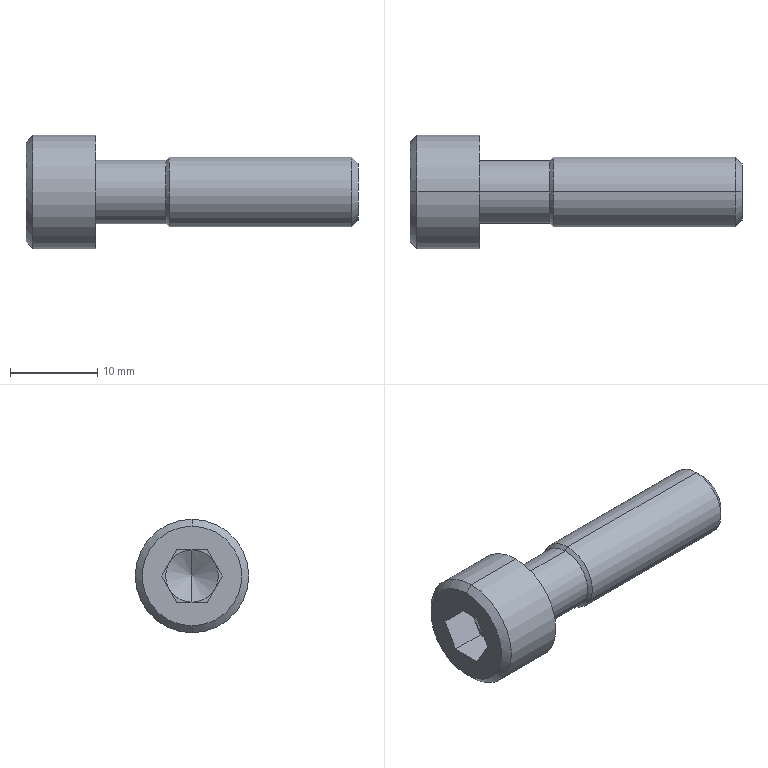Part | STEP file | 0244_Z_017_SCBS8-30_1 | 1 solid | 29 faces | box 38 x 13 x 13 mm | volume 2334 mm3 | plane 15 | cone 8 | cylinder 6 | commonest cylinder face diameters 7.232 x2 8 x2 13 x2